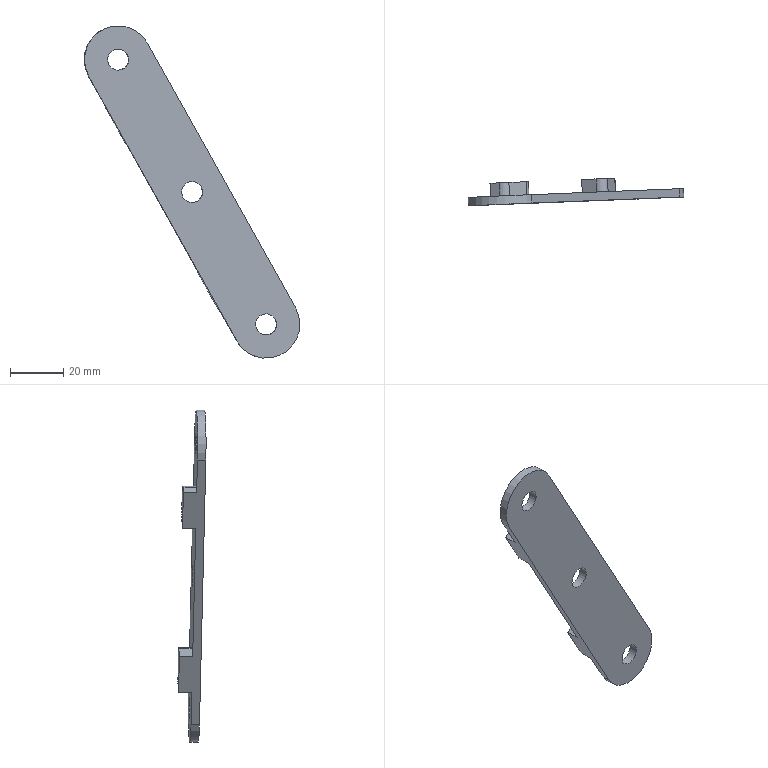Part | NX | features MG0330 trunion parts 24(steering fork) 2 | 1 solid | 21 faces | box 81.261 x 10.57 x 125.154 mm | volume 11578 mm3 | plane 12 | cylinder 9 | commonest cylinder face diameters 6 x4 7.938 x3 25.4 x2
STEP:
#1=CARTESIAN_POINT('',(621.854,-233.442,-30.331));
#2=VERTEX_POINT('',#1);
#3=CARTESIAN_POINT('',(627.267,-233.207,-27.3));
#4=VERTEX_POINT('',#3);
#5=CARTESIAN_POINT('',(621.854,-233.442,-30.331));
#6=DIRECTION('',(0.8719,0.03772,0.4882));
#7=VECTOR('',#6,1000.);
#8=LINE('',#5,#7);
#9=EDGE_CURVE('',#2,#4,#8,.T.);
#10=ORIENTED_EDGE('',*,*,#9,.F.);
#11=CARTESIAN_POINT('',(594.883,-234.609,17.931));
#12=VERTEX_POINT('',#11);
#13=CARTESIAN_POINT('',(636.242,-232.819,-56.077));
#14=DIRECTION('',(-0.4877,-0.0211,0.8727));
#15=VECTOR('',#14,1000.);
#16=LINE('',#13,#15);
#17=EDGE_CURVE('',#2,#12,#16,.T.);
#18=ORIENTED_EDGE('',*,*,#17,.T.);
#19=CARTESIAN_POINT('',(600.295,-234.374,20.962));
#20=VERTEX_POINT('',#19);
#21=CARTESIAN_POINT('',(594.883,-234.609,17.931));
#22=DIRECTION('',(0.8719,0.03772,0.4882));
#23=VECTOR('',#22,1000.);
#24=LINE('',#21,#23);
#25=EDGE_CURVE('',#20,#12,#24,.F.);
#26=ORIENTED_EDGE('',*,*,#25,.F.);
#27=CARTESIAN_POINT('',(601.041,-234.342,25.607));
#28=VERTEX_POINT('',#27);
#29=CARTESIAN_POINT('',(598.832,-234.438,23.58));
#30=DIRECTION('',(0.04322,-0.9991,0.));
#31=DIRECTION('',(-0.4877,-0.0211,0.8727));
#32=AXIS2_PLACEMENT_3D('',#29,#30,#31);
#33=CIRCLE('',#32,3.);
#34=EDGE_CURVE('',#20,#28,#33,.T.);
#35=ORIENTED_EDGE('',*,*,#34,.T.);
#36=CARTESIAN_POINT('',(594.449,-234.627,32.802));
#37=VERTEX_POINT('',#36);
#38=CARTESIAN_POINT('',(603.602,-234.231,22.813));
#39=DIRECTION('',(-0.6753,-0.02921,0.737));
#40=VECTOR('',#39,1000.);
#41=LINE('',#38,#40);
#42=EDGE_CURVE('',#28,#37,#41,.T.);
#43=ORIENTED_EDGE('',*,*,#42,.T.);
#44=CARTESIAN_POINT('',(590.777,-234.786,33.393));
#45=VERTEX_POINT('',#44);
#46=CARTESIAN_POINT('',(592.24,-234.723,30.775));
#47=DIRECTION('',(0.04322,-0.9991,0.));
#48=DIRECTION('',(-0.4877,-0.0211,0.8727));
#49=AXIS2_PLACEMENT_3D('',#46,#47,#48);
#50=CIRCLE('',#49,3.);
#51=EDGE_CURVE('',#37,#45,#50,.T.);
#52=ORIENTED_EDGE('',*,*,#51,.T.);
#53=CARTESIAN_POINT('',(587.322,-234.936,31.459));
#54=VERTEX_POINT('',#53);
#55=CARTESIAN_POINT('',(592.847,-234.697,34.552));
#56=DIRECTION('',(-0.8719,-0.03772,-0.4882));
#57=VECTOR('',#56,1000.);
#58=LINE('',#55,#57);
#59=EDGE_CURVE('',#54,#45,#58,.F.);
#60=ORIENTED_EDGE('',*,*,#59,.F.);
#61=CARTESIAN_POINT('',(580.494,-235.231,43.677));
#62=VERTEX_POINT('',#61);
#63=CARTESIAN_POINT('',(636.242,-232.819,-56.077));
#64=DIRECTION('',(-0.4877,-0.0211,0.8727));
#65=VECTOR('',#64,1000.);
#66=LINE('',#63,#65);
#67=EDGE_CURVE('',#54,#62,#66,.T.);
#68=ORIENTED_EDGE('',*,*,#67,.T.);
#69=CARTESIAN_POINT('',(602.641,-234.273,56.077));
#70=VERTEX_POINT('',#69);
#71=CARTESIAN_POINT('',(591.568,-234.752,49.877));
#72=DIRECTION('',(-0.04322,0.9991,0.));
#73=DIRECTION('',(0.8719,0.03772,0.4882));
#74=AXIS2_PLACEMENT_3D('',#71,#72,#73);
#75=CIRCLE('',#74,12.7);
#76=EDGE_CURVE('',#62,#70,#75,.T.);
#77=ORIENTED_EDGE('',*,*,#76,.T.);
#78=CARTESIAN_POINT('',(658.389,-231.861,-43.677));
#79=VERTEX_POINT('',#78);
#80=CARTESIAN_POINT('',(658.389,-231.861,-43.677));
#81=DIRECTION('',(0.4877,0.0211,-0.8727));
#82=VECTOR('',#81,1000.);
#83=LINE('',#80,#82);
#84=EDGE_CURVE('',#70,#79,#83,.T.);
#85=ORIENTED_EDGE('',*,*,#84,.T.);
#86=CARTESIAN_POINT('',(636.242,-232.819,-56.077));
#87=VERTEX_POINT('',#86);
#88=CARTESIAN_POINT('',(647.315,-232.34,-49.877));
#89=DIRECTION('',(-0.04322,0.9991,0.));
#90=DIRECTION('',(0.8719,0.03772,0.4882));
#91=AXIS2_PLACEMENT_3D('',#88,#89,#90);
#92=CIRCLE('',#91,12.7);
#93=EDGE_CURVE('',#79,#87,#92,.T.);
#94=ORIENTED_EDGE('',*,*,#93,.T.);
#95=CARTESIAN_POINT('',(629.414,-233.115,-43.859));
#96=VERTEX_POINT('',#95);
#97=CARTESIAN_POINT('',(636.242,-232.819,-56.077));
#98=DIRECTION('',(-0.4877,-0.0211,0.8727));
#99=VECTOR('',#98,1000.);
#100=LINE('',#97,#99);
#101=EDGE_CURVE('',#87,#96,#100,.T.);
#102=ORIENTED_EDGE('',*,*,#101,.T.);
#103=CARTESIAN_POINT('',(632.868,-232.965,-41.924));
#104=VERTEX_POINT('',#103);
#105=CARTESIAN_POINT('',(634.938,-232.876,-40.766));
#106=DIRECTION('',(-0.8719,-0.03772,-0.4882));
#107=VECTOR('',#106,1000.);
#108=LINE('',#105,#107);
#109=EDGE_CURVE('',#104,#96,#108,.T.);
#110=ORIENTED_EDGE('',*,*,#109,.F.);
#111=CARTESIAN_POINT('',(634.287,-232.904,-38.483));
#112=VERTEX_POINT('',#111);
#113=CARTESIAN_POINT('',(631.405,-233.028,-39.306));
#114=DIRECTION('',(-0.04322,0.9991,0.));
#115=DIRECTION('',(-0.9991,-0.04322,0.));
#116=AXIS2_PLACEMENT_3D('',#113,#114,#115);
#117=CIRCLE('',#116,3.);
#118=EDGE_CURVE('',#104,#112,#117,.F.);
#119=ORIENTED_EDGE('',*,*,#118,.T.);
#120=CARTESIAN_POINT('',(631.612,-233.019,-29.095));
#121=VERTEX_POINT('',#120);
#122=CARTESIAN_POINT('',(633.424,-232.941,-35.455));
#123=DIRECTION('',(0.274,0.01186,-0.9616));
#124=VECTOR('',#123,1000.);
#125=LINE('',#122,#124);
#126=EDGE_CURVE('',#121,#112,#125,.T.);
#127=ORIENTED_EDGE('',*,*,#126,.F.);
#128=CARTESIAN_POINT('',(628.73,-233.144,-29.918));
#129=DIRECTION('',(-0.04322,0.9991,0.));
#130=DIRECTION('',(-0.9991,-0.04322,0.));
#131=AXIS2_PLACEMENT_3D('',#128,#129,#130);
#132=CIRCLE('',#131,3.);
#133=EDGE_CURVE('',#121,#4,#132,.F.);
#134=ORIENTED_EDGE('',*,*,#133,.T.);
#135=EDGE_LOOP('',(#10,#18,#26,#35,#43,#52,#60,#68,#77,#85,#94,#102,#110,#119,#127,#134));
#136=FACE_BOUND('',#135,.T.);
#137=CARTESIAN_POINT('',(595.028,-234.602,51.814));
#138=VERTEX_POINT('',#137);
#139=CARTESIAN_POINT('',(591.568,-234.752,49.877));
#140=DIRECTION('',(-0.04322,0.9991,0.));
#141=DIRECTION('',(0.8719,0.03772,0.4882));
#142=AXIS2_PLACEMENT_3D('',#139,#140,#141);
#143=CIRCLE('',#142,3.969);
#144=EDGE_CURVE('',#138,#138,#143,.T.);
#145=ORIENTED_EDGE('',*,*,#144,.F.);
#146=EDGE_LOOP('',(#145));
#147=FACE_BOUND('',#146,.T.);
#148=CARTESIAN_POINT('',(622.902,-233.396,1.937));
#149=VERTEX_POINT('',#148);
#150=CARTESIAN_POINT('',(619.442,-233.546,0.));
#151=DIRECTION('',(-0.04322,0.9991,0.));
#152=DIRECTION('',(0.8719,0.03772,0.4882));
#153=AXIS2_PLACEMENT_3D('',#150,#151,#152);
#154=CIRCLE('',#153,3.969);
#155=EDGE_CURVE('',#149,#149,#154,.T.);
#156=ORIENTED_EDGE('',*,*,#155,.F.);
#157=EDGE_LOOP('',(#156));
#158=FACE_BOUND('',#157,.T.);
#159=CARTESIAN_POINT('',(650.776,-232.19,-47.94));
#160=VERTEX_POINT('',#159);
#161=CARTESIAN_POINT('',(647.315,-232.34,-49.877));
#162=DIRECTION('',(-0.04322,0.9991,0.));
#163=DIRECTION('',(0.8719,0.03772,0.4882));
#164=AXIS2_PLACEMENT_3D('',#161,#162,#163);
#165=CIRCLE('',#164,3.969);
#166=EDGE_CURVE('',#160,#160,#165,.T.);
#167=ORIENTED_EDGE('',*,*,#166,.F.);
#168=EDGE_LOOP('',(#167));
#169=FACE_BOUND('',#168,.T.);
#170=CARTESIAN_POINT('',(647.315,-232.34,-49.877));
#171=DIRECTION('',(-0.04322,0.9991,0.));
#172=DIRECTION('',(0.8719,0.03772,0.4882));
#173=AXIS2_PLACEMENT_3D('',#170,#171,#172);
#174=PLANE('',#173);
#175=ADVANCED_FACE('',(#136,#147,#158,#169),#174,.T.);
#176=CARTESIAN_POINT('',(658.526,-235.033,-43.677));
#177=VERTEX_POINT('',#176);
#178=CARTESIAN_POINT('',(636.379,-235.991,-56.077));
#179=VERTEX_POINT('',#178);
#180=CARTESIAN_POINT('',(647.453,-235.512,-49.877));
#181=DIRECTION('',(-0.04322,0.9991,0.));
#182=DIRECTION('',(0.8719,0.03772,0.4882));
#183=AXIS2_PLACEMENT_3D('',#180,#181,#182);
#184=CIRCLE('',#183,12.7);
#185=EDGE_CURVE('',#177,#179,#184,.T.);
#186=ORIENTED_EDGE('',*,*,#185,.F.);
#187=CARTESIAN_POINT('',(602.778,-237.445,56.077));
#188=VERTEX_POINT('',#187);
#189=CARTESIAN_POINT('',(658.526,-235.033,-43.677));
#190=DIRECTION('',(0.4877,0.0211,-0.8727));
#191=VECTOR('',#190,1000.);
#192=LINE('',#189,#191);
#193=EDGE_CURVE('',#188,#177,#192,.T.);
#194=ORIENTED_EDGE('',*,*,#193,.F.);
#195=CARTESIAN_POINT('',(580.631,-238.403,43.677));
#196=VERTEX_POINT('',#195);
#197=CARTESIAN_POINT('',(591.705,-237.924,49.877));
#198=DIRECTION('',(-0.04322,0.9991,0.));
#199=DIRECTION('',(0.8719,0.03772,0.4882));
#200=AXIS2_PLACEMENT_3D('',#197,#198,#199);
#201=CIRCLE('',#200,12.7);
#202=EDGE_CURVE('',#196,#188,#201,.T.);
#203=ORIENTED_EDGE('',*,*,#202,.F.);
#204=CARTESIAN_POINT('',(636.379,-235.991,-56.077));
#205=DIRECTION('',(-0.4877,-0.0211,0.8727));
#206=VECTOR('',#205,1000.);
#207=LINE('',#204,#206);
#208=EDGE_CURVE('',#179,#196,#207,.T.);
#209=ORIENTED_EDGE('',*,*,#208,.F.);
#210=EDGE_LOOP('',(#186,#194,#203,#209));
#211=FACE_BOUND('',#210,.T.);
#212=CARTESIAN_POINT('',(623.039,-236.568,1.937));
#213=VERTEX_POINT('',#212);
#214=CARTESIAN_POINT('',(619.579,-236.718,0.));
#215=DIRECTION('',(-0.04322,0.9991,0.));
#216=DIRECTION('',(0.8719,0.03772,0.4882));
#217=AXIS2_PLACEMENT_3D('',#214,#215,#216);
#218=CIRCLE('',#217,3.969);
#219=EDGE_CURVE('',#213,#213,#218,.T.);
#220=ORIENTED_EDGE('',*,*,#219,.T.);
#221=EDGE_LOOP('',(#220));
#222=FACE_BOUND('',#221,.T.);
#223=CARTESIAN_POINT('',(595.165,-237.774,51.814));
#224=VERTEX_POINT('',#223);
#225=CARTESIAN_POINT('',(591.705,-237.924,49.877));
#226=DIRECTION('',(-0.04322,0.9991,0.));
#227=DIRECTION('',(0.8719,0.03772,0.4882));
#228=AXIS2_PLACEMENT_3D('',#225,#226,#227);
#229=CIRCLE('',#228,3.969);
#230=EDGE_CURVE('',#224,#224,#229,.T.);
#231=ORIENTED_EDGE('',*,*,#230,.T.);
#232=EDGE_LOOP('',(#231));
#233=FACE_BOUND('',#232,.T.);
#234=CARTESIAN_POINT('',(650.913,-235.362,-47.94));
#235=VERTEX_POINT('',#234);
#236=CARTESIAN_POINT('',(647.453,-235.512,-49.877));
#237=DIRECTION('',(-0.04322,0.9991,0.));
#238=DIRECTION('',(0.8719,0.03772,0.4882));
#239=AXIS2_PLACEMENT_3D('',#236,#237,#238);
#240=CIRCLE('',#239,3.969);
#241=EDGE_CURVE('',#235,#235,#240,.T.);
#242=ORIENTED_EDGE('',*,*,#241,.T.);
#243=EDGE_LOOP('',(#242));
#244=FACE_BOUND('',#243,.T.);
#245=CARTESIAN_POINT('',(647.453,-235.512,-49.877));
#246=DIRECTION('',(-0.04322,0.9991,0.));
#247=DIRECTION('',(0.8719,0.03772,0.4882));
#248=AXIS2_PLACEMENT_3D('',#245,#246,#247);
#249=PLANE('',#248);
#250=ADVANCED_FACE('',(#211,#222,#233,#244),#249,.F.);
#251=ORIENTED_EDGE('',*,*,#185,.T.);
#252=CARTESIAN_POINT('',(636.242,-232.819,-56.077));
#253=DIRECTION('',(0.04322,-0.9991,0.));
#254=VECTOR('',#253,1000.);
#255=LINE('',#252,#254);
#256=EDGE_CURVE('',#87,#179,#255,.T.);
#257=ORIENTED_EDGE('',*,*,#256,.F.);
#258=ORIENTED_EDGE('',*,*,#93,.F.);
#259=CARTESIAN_POINT('',(658.389,-231.861,-43.677));
#260=DIRECTION('',(0.04322,-0.9991,0.));
#261=VECTOR('',#260,1000.);
#262=LINE('',#259,#261);
#263=EDGE_CURVE('',#79,#177,#262,.T.);
#264=ORIENTED_EDGE('',*,*,#263,.T.);
#265=EDGE_LOOP('',(#251,#257,#258,#264));
#266=FACE_BOUND('',#265,.T.);
#267=CARTESIAN_POINT('',(647.315,-232.34,-49.877));
#268=DIRECTION('',(0.04322,-0.9991,0.));
#269=DIRECTION('',(-0.8719,-0.03772,-0.4882));
#270=AXIS2_PLACEMENT_3D('',#267,#268,#269);
#271=CYLINDRICAL_SURFACE('',#270,12.7);
#272=ADVANCED_FACE('',(#266),#271,.T.);
#273=ORIENTED_EDGE('',*,*,#208,.T.);
#274=CARTESIAN_POINT('',(580.494,-235.231,43.677));
#275=DIRECTION('',(0.04322,-0.9991,0.));
#276=VECTOR('',#275,1000.);
#277=LINE('',#274,#276);
#278=EDGE_CURVE('',#62,#196,#277,.T.);
#279=ORIENTED_EDGE('',*,*,#278,.F.);
#280=ORIENTED_EDGE('',*,*,#67,.F.);
#281=CARTESIAN_POINT('',(587.106,-229.94,31.459));
#282=VERTEX_POINT('',#281);
#283=CARTESIAN_POINT('',(587.106,-229.94,31.459));
#284=DIRECTION('',(0.04322,-0.9991,0.));
#285=VECTOR('',#284,1000.);
#286=LINE('',#283,#285);
#287=EDGE_CURVE('',#54,#282,#286,.F.);
#288=ORIENTED_EDGE('',*,*,#287,.T.);
#289=CARTESIAN_POINT('',(594.666,-229.613,17.931));
#290=VERTEX_POINT('',#289);
#291=CARTESIAN_POINT('',(587.106,-229.94,31.459));
#292=DIRECTION('',(0.4877,0.0211,-0.8727));
#293=VECTOR('',#292,1000.);
#294=LINE('',#291,#293);
#295=EDGE_CURVE('',#290,#282,#294,.F.);
#296=ORIENTED_EDGE('',*,*,#295,.F.);
#297=CARTESIAN_POINT('',(594.666,-229.613,17.931));
#298=DIRECTION('',(0.04322,-0.9991,0.));
#299=VECTOR('',#298,1000.);
#300=LINE('',#297,#299);
#301=EDGE_CURVE('',#12,#290,#300,.F.);
#302=ORIENTED_EDGE('',*,*,#301,.F.);
#303=ORIENTED_EDGE('',*,*,#17,.F.);
#304=CARTESIAN_POINT('',(621.638,-228.446,-30.331));
#305=VERTEX_POINT('',#304);
#306=CARTESIAN_POINT('',(621.638,-228.446,-30.331));
#307=DIRECTION('',(0.04322,-0.9991,0.));
#308=VECTOR('',#307,1000.);
#309=LINE('',#306,#308);
#310=EDGE_CURVE('',#305,#2,#309,.T.);
#311=ORIENTED_EDGE('',*,*,#310,.F.);
#312=CARTESIAN_POINT('',(629.198,-228.119,-43.859));
#313=VERTEX_POINT('',#312);
#314=CARTESIAN_POINT('',(629.198,-228.119,-43.859));
#315=DIRECTION('',(-0.4877,-0.0211,0.8727));
#316=VECTOR('',#315,1000.);
#317=LINE('',#314,#316);
#318=EDGE_CURVE('',#313,#305,#317,.T.);
#319=ORIENTED_EDGE('',*,*,#318,.F.);
#320=CARTESIAN_POINT('',(629.198,-228.119,-43.859));
#321=DIRECTION('',(0.04322,-0.9991,0.));
#322=VECTOR('',#321,1000.);
#323=LINE('',#320,#322);
#324=EDGE_CURVE('',#313,#96,#323,.T.);
#325=ORIENTED_EDGE('',*,*,#324,.T.);
#326=ORIENTED_EDGE('',*,*,#101,.F.);
#327=ORIENTED_EDGE('',*,*,#256,.T.);
#328=EDGE_LOOP('',(#273,#279,#280,#288,#296,#302,#303,#311,#319,#325,#326,#327));
#329=FACE_BOUND('',#328,.T.);
#330=CARTESIAN_POINT('',(636.242,-232.819,-56.077));
#331=DIRECTION('',(0.8719,0.03772,0.4882));
#332=DIRECTION('',(-0.4877,-0.0211,0.8727));
#333=AXIS2_PLACEMENT_3D('',#330,#331,#332);
#334=PLANE('',#333);
#335=ADVANCED_FACE('',(#329),#334,.F.);
#336=ORIENTED_EDGE('',*,*,#202,.T.);
#337=CARTESIAN_POINT('',(602.641,-234.273,56.077));
#338=DIRECTION('',(0.04322,-0.9991,0.));
#339=VECTOR('',#338,1000.);
#340=LINE('',#337,#339);
#341=EDGE_CURVE('',#70,#188,#340,.T.);
#342=ORIENTED_EDGE('',*,*,#341,.F.);
#343=ORIENTED_EDGE('',*,*,#76,.F.);
#344=ORIENTED_EDGE('',*,*,#278,.T.);
#345=EDGE_LOOP('',(#336,#342,#343,#344));
#346=FACE_BOUND('',#345,.T.);
#347=CARTESIAN_POINT('',(591.568,-234.752,49.877));
#348=DIRECTION('',(0.04322,-0.9991,0.));
#349=DIRECTION('',(-0.8719,-0.03772,-0.4882));
#350=AXIS2_PLACEMENT_3D('',#347,#348,#349);
#351=CYLINDRICAL_SURFACE('',#350,12.7);
#352=ADVANCED_FACE('',(#346),#351,.T.);
#353=ORIENTED_EDGE('',*,*,#193,.T.);
#354=ORIENTED_EDGE('',*,*,#263,.F.);
#355=ORIENTED_EDGE('',*,*,#84,.F.);
#356=ORIENTED_EDGE('',*,*,#341,.T.);
#357=EDGE_LOOP('',(#353,#354,#355,#356));
#358=FACE_BOUND('',#357,.T.);
#359=CARTESIAN_POINT('',(658.389,-231.861,-43.677));
#360=DIRECTION('',(-0.8719,-0.03772,-0.4882));
#361=DIRECTION('',(0.4877,0.0211,-0.8727));
#362=AXIS2_PLACEMENT_3D('',#359,#360,#361);
#363=PLANE('',#362);
#364=ADVANCED_FACE('',(#358),#363,.F.);
#365=ORIENTED_EDGE('',*,*,#155,.T.);
#366=EDGE_LOOP('',(#365));
#367=FACE_BOUND('',#366,.T.);
#368=ORIENTED_EDGE('',*,*,#219,.F.);
#369=EDGE_LOOP('',(#368));
#370=FACE_BOUND('',#369,.T.);
#371=CARTESIAN_POINT('',(619.442,-233.546,0.));
#372=DIRECTION('',(0.04322,-0.9991,0.));
#373=DIRECTION('',(-0.8719,-0.03772,-0.4882));
#374=AXIS2_PLACEMENT_3D('',#371,#372,#373);
#375=CYLINDRICAL_SURFACE('',#374,3.969);
#376=ADVANCED_FACE('',(#367,#370),#375,.F.);
#377=ORIENTED_EDGE('',*,*,#144,.T.);
#378=EDGE_LOOP('',(#377));
#379=FACE_BOUND('',#378,.T.);
#380=ORIENTED_EDGE('',*,*,#230,.F.);
#381=EDGE_LOOP('',(#380));
#382=FACE_BOUND('',#381,.T.);
#383=CARTESIAN_POINT('',(591.568,-234.752,49.877));
#384=DIRECTION('',(0.04322,-0.9991,0.));
#385=DIRECTION('',(-0.8719,-0.03772,-0.4882));
#386=AXIS2_PLACEMENT_3D('',#383,#384,#385);
#387=CYLINDRICAL_SURFACE('',#386,3.969);
#388=ADVANCED_FACE('',(#379,#382),#387,.F.);
#389=ORIENTED_EDGE('',*,*,#166,.T.);
#390=EDGE_LOOP('',(#389));
#391=FACE_BOUND('',#390,.T.);
#392=ORIENTED_EDGE('',*,*,#241,.F.);
#393=EDGE_LOOP('',(#392));
#394=FACE_BOUND('',#393,.T.);
#395=CARTESIAN_POINT('',(647.315,-232.34,-49.877));
#396=DIRECTION('',(0.04322,-0.9991,0.));
#397=DIRECTION('',(-0.8719,-0.03772,-0.4882));
#398=AXIS2_PLACEMENT_3D('',#395,#396,#397);
#399=CYLINDRICAL_SURFACE('',#398,3.969);
#400=ADVANCED_FACE('',(#391,#394),#399,.F.);
#401=CARTESIAN_POINT('',(600.079,-229.379,20.962));
#402=VERTEX_POINT('',#401);
#403=CARTESIAN_POINT('',(594.666,-229.613,17.931));
#404=DIRECTION('',(0.8719,0.03772,0.4882));
#405=VECTOR('',#404,1000.);
#406=LINE('',#403,#405);
#407=EDGE_CURVE('',#402,#290,#406,.F.);
#408=ORIENTED_EDGE('',*,*,#407,.F.);
#409=CARTESIAN_POINT('',(600.079,-229.379,20.962));
#410=DIRECTION('',(0.04322,-0.9991,0.));
#411=VECTOR('',#410,1000.);
#412=LINE('',#409,#411);
#413=EDGE_CURVE('',#402,#20,#412,.T.);
#414=ORIENTED_EDGE('',*,*,#413,.T.);
#415=ORIENTED_EDGE('',*,*,#25,.T.);
#416=ORIENTED_EDGE('',*,*,#301,.T.);
#417=EDGE_LOOP('',(#408,#414,#415,#416));
#418=FACE_BOUND('',#417,.T.);
#419=CARTESIAN_POINT('',(594.666,-229.613,17.931));
#420=DIRECTION('',(0.4877,0.0211,-0.8727));
#421=DIRECTION('',(-0.8729,0.,-0.4878));
#422=AXIS2_PLACEMENT_3D('',#419,#420,#421);
#423=PLANE('',#422);
#424=ADVANCED_FACE('',(#418),#423,.T.);
#425=CARTESIAN_POINT('',(600.825,-229.347,25.607));
#426=VERTEX_POINT('',#425);
#427=CARTESIAN_POINT('',(594.233,-229.632,32.802));
#428=VERTEX_POINT('',#427);
#429=CARTESIAN_POINT('',(603.386,-229.236,22.813));
#430=DIRECTION('',(-0.6753,-0.02921,0.737));
#431=VECTOR('',#430,1000.);
#432=LINE('',#429,#431);
#433=EDGE_CURVE('',#426,#428,#432,.T.);
#434=ORIENTED_EDGE('',*,*,#433,.T.);
#435=CARTESIAN_POINT('',(594.233,-229.632,32.802));
#436=DIRECTION('',(0.04322,-0.9991,0.));
#437=VECTOR('',#436,1000.);
#438=LINE('',#435,#437);
#439=EDGE_CURVE('',#428,#37,#438,.T.);
#440=ORIENTED_EDGE('',*,*,#439,.T.);
#441=ORIENTED_EDGE('',*,*,#42,.F.);
#442=CARTESIAN_POINT('',(600.825,-229.347,25.607));
#443=DIRECTION('',(0.04322,-0.9991,0.));
#444=VECTOR('',#443,1000.);
#445=LINE('',#442,#444);
#446=EDGE_CURVE('',#28,#426,#445,.F.);
#447=ORIENTED_EDGE('',*,*,#446,.T.);
#448=EDGE_LOOP('',(#434,#440,#441,#447));
#449=FACE_BOUND('',#448,.T.);
#450=CARTESIAN_POINT('',(603.386,-229.236,22.813));
#451=DIRECTION('',(0.7363,0.03186,0.6759));
#452=DIRECTION('',(0.6762,0.,-0.7367));
#453=AXIS2_PLACEMENT_3D('',#450,#451,#452);
#454=PLANE('',#453);
#455=ADVANCED_FACE('',(#449),#454,.T.);
#456=ORIENTED_EDGE('',*,*,#59,.T.);
#457=CARTESIAN_POINT('',(590.561,-229.791,33.393));
#458=VERTEX_POINT('',#457);
#459=CARTESIAN_POINT('',(590.561,-229.791,33.393));
#460=DIRECTION('',(0.04322,-0.9991,0.));
#461=VECTOR('',#460,1000.);
#462=LINE('',#459,#461);
#463=EDGE_CURVE('',#45,#458,#462,.F.);
#464=ORIENTED_EDGE('',*,*,#463,.T.);
#465=CARTESIAN_POINT('',(592.63,-229.701,34.552));
#466=DIRECTION('',(-0.8719,-0.03772,-0.4882));
#467=VECTOR('',#466,1000.);
#468=LINE('',#465,#467);
#469=EDGE_CURVE('',#282,#458,#468,.F.);
#470=ORIENTED_EDGE('',*,*,#469,.F.);
#471=ORIENTED_EDGE('',*,*,#287,.F.);
#472=EDGE_LOOP('',(#456,#464,#470,#471));
#473=FACE_BOUND('',#472,.T.);
#474=CARTESIAN_POINT('',(592.63,-229.701,34.552));
#475=DIRECTION('',(-0.4877,-0.0211,0.8727));
#476=DIRECTION('',(0.8729,0.,0.4878));
#477=AXIS2_PLACEMENT_3D('',#474,#475,#476);
#478=PLANE('',#477);
#479=ADVANCED_FACE('',(#473),#478,.T.);
#480=ORIENTED_EDGE('',*,*,#469,.T.);
#481=CARTESIAN_POINT('',(592.024,-229.727,30.775));
#482=DIRECTION('',(0.04322,-0.9991,0.));
#483=DIRECTION('',(-0.4877,-0.0211,0.8727));
#484=AXIS2_PLACEMENT_3D('',#481,#482,#483);
#485=CIRCLE('',#484,3.);
#486=EDGE_CURVE('',#458,#428,#485,.F.);
#487=ORIENTED_EDGE('',*,*,#486,.T.);
#488=ORIENTED_EDGE('',*,*,#433,.F.);
#489=CARTESIAN_POINT('',(598.616,-229.442,23.58));
#490=DIRECTION('',(0.04322,-0.9991,0.));
#491=DIRECTION('',(-0.4877,-0.0211,0.8727));
#492=AXIS2_PLACEMENT_3D('',#489,#490,#491);
#493=CIRCLE('',#492,3.);
#494=EDGE_CURVE('',#426,#402,#493,.F.);
#495=ORIENTED_EDGE('',*,*,#494,.T.);
#496=ORIENTED_EDGE('',*,*,#407,.T.);
#497=ORIENTED_EDGE('',*,*,#295,.T.);
#498=EDGE_LOOP('',(#480,#487,#488,#495,#496,#497));
#499=FACE_BOUND('',#498,.T.);
#500=CARTESIAN_POINT('',(11.027,-254.864,0.));
#501=DIRECTION('',(0.04322,-0.9991,0.));
#502=DIRECTION('',(0.9991,0.04322,0.));
#503=AXIS2_PLACEMENT_3D('',#500,#501,#502);
#504=PLANE('',#503);
#505=ADVANCED_FACE('',(#499),#504,.F.);
#506=ORIENTED_EDGE('',*,*,#486,.F.);
#507=ORIENTED_EDGE('',*,*,#463,.F.);
#508=ORIENTED_EDGE('',*,*,#51,.F.);
#509=ORIENTED_EDGE('',*,*,#439,.F.);
#510=EDGE_LOOP('',(#506,#507,#508,#509));
#511=FACE_BOUND('',#510,.T.);
#512=CARTESIAN_POINT('',(592.024,-229.727,30.775));
#513=DIRECTION('',(0.04322,-0.9991,0.));
#514=DIRECTION('',(-0.4877,-0.0211,0.8727));
#515=AXIS2_PLACEMENT_3D('',#512,#513,#514);
#516=CYLINDRICAL_SURFACE('',#515,3.);
#517=ADVANCED_FACE('',(#511),#516,.T.);
#518=ORIENTED_EDGE('',*,*,#494,.F.);
#519=ORIENTED_EDGE('',*,*,#446,.F.);
#520=ORIENTED_EDGE('',*,*,#34,.F.);
#521=ORIENTED_EDGE('',*,*,#413,.F.);
#522=EDGE_LOOP('',(#518,#519,#520,#521));
#523=FACE_BOUND('',#522,.T.);
#524=CARTESIAN_POINT('',(598.616,-229.442,23.58));
#525=DIRECTION('',(0.04322,-0.9991,0.));
#526=DIRECTION('',(-0.4877,-0.0211,0.8727));
#527=AXIS2_PLACEMENT_3D('',#524,#525,#526);
#528=CYLINDRICAL_SURFACE('',#527,3.);
#529=ADVANCED_FACE('',(#523),#528,.T.);
#530=ORIENTED_EDGE('',*,*,#9,.T.);
#531=CARTESIAN_POINT('',(627.05,-228.212,-27.3));
#532=VERTEX_POINT('',#531);
#533=CARTESIAN_POINT('',(627.05,-228.212,-27.3));
#534=DIRECTION('',(0.04322,-0.9991,0.));
#535=VECTOR('',#534,1000.);
#536=LINE('',#533,#535);
#537=EDGE_CURVE('',#4,#532,#536,.F.);
#538=ORIENTED_EDGE('',*,*,#537,.T.);
#539=CARTESIAN_POINT('',(621.638,-228.446,-30.331));
#540=DIRECTION('',(0.8719,0.03772,0.4882));
#541=VECTOR('',#540,1000.);
#542=LINE('',#539,#541);
#543=EDGE_CURVE('',#305,#532,#542,.T.);
#544=ORIENTED_EDGE('',*,*,#543,.F.);
#545=ORIENTED_EDGE('',*,*,#310,.T.);
#546=EDGE_LOOP('',(#530,#538,#544,#545));
#547=FACE_BOUND('',#546,.T.);
#548=CARTESIAN_POINT('',(621.638,-228.446,-30.331));
#549=DIRECTION('',(0.4877,0.0211,-0.8727));
#550=DIRECTION('',(-0.8729,0.,-0.4878));
#551=AXIS2_PLACEMENT_3D('',#548,#549,#550);
#552=PLANE('',#551);
#553=ADVANCED_FACE('',(#547),#552,.F.);
#554=CARTESIAN_POINT('',(631.396,-228.024,-29.095));
#555=VERTEX_POINT('',#554);
#556=CARTESIAN_POINT('',(634.071,-227.908,-38.483));
#557=VERTEX_POINT('',#556);
#558=CARTESIAN_POINT('',(630.357,-228.069,-25.449));
#559=DIRECTION('',(0.274,0.01186,-0.9616));
#560=VECTOR('',#559,1000.);
#561=LINE('',#558,#560);
#562=EDGE_CURVE('',#555,#557,#561,.T.);
#563=ORIENTED_EDGE('',*,*,#562,.F.);
#564=CARTESIAN_POINT('',(631.396,-228.024,-29.095));
#565=DIRECTION('',(0.04322,-0.9991,0.));
#566=VECTOR('',#565,1000.);
#567=LINE('',#564,#566);
#568=EDGE_CURVE('',#555,#121,#567,.T.);
#569=ORIENTED_EDGE('',*,*,#568,.T.);
#570=ORIENTED_EDGE('',*,*,#126,.T.);
#571=CARTESIAN_POINT('',(634.071,-227.908,-38.483));
#572=DIRECTION('',(0.04322,-0.9991,0.));
#573=VECTOR('',#572,1000.);
#574=LINE('',#571,#573);
#575=EDGE_CURVE('',#112,#557,#574,.F.);
#576=ORIENTED_EDGE('',*,*,#575,.T.);
#577=EDGE_LOOP('',(#563,#569,#570,#576));
#578=FACE_BOUND('',#577,.T.);
#579=CARTESIAN_POINT('',(633.208,-227.946,-35.455));
#580=DIRECTION('',(-0.9607,-0.04157,-0.2743));
#581=DIRECTION('',(-0.2745,0.,0.9616));
#582=AXIS2_PLACEMENT_3D('',#579,#580,#581);
#583=PLANE('',#582);
#584=ADVANCED_FACE('',(#578),#583,.F.);
#585=CARTESIAN_POINT('',(632.652,-227.97,-41.924));
#586=VERTEX_POINT('',#585);
#587=CARTESIAN_POINT('',(634.722,-227.88,-40.766));
#588=DIRECTION('',(-0.8719,-0.03772,-0.4882));
#589=VECTOR('',#588,1000.);
#590=LINE('',#587,#589);
#591=EDGE_CURVE('',#586,#313,#590,.T.);
#592=ORIENTED_EDGE('',*,*,#591,.F.);
#593=CARTESIAN_POINT('',(632.652,-227.97,-41.924));
#594=DIRECTION('',(0.04322,-0.9991,0.));
#595=VECTOR('',#594,1000.);
#596=LINE('',#593,#595);
#597=EDGE_CURVE('',#586,#104,#596,.T.);
#598=ORIENTED_EDGE('',*,*,#597,.T.);
#599=ORIENTED_EDGE('',*,*,#109,.T.);
#600=ORIENTED_EDGE('',*,*,#324,.F.);
#601=EDGE_LOOP('',(#592,#598,#599,#600));
#602=FACE_BOUND('',#601,.T.);
#603=CARTESIAN_POINT('',(634.722,-227.88,-40.766));
#604=DIRECTION('',(-0.4877,-0.0211,0.8727));
#605=DIRECTION('',(0.8729,0.,0.4878));
#606=AXIS2_PLACEMENT_3D('',#603,#604,#605);
#607=PLANE('',#606);
#608=ADVANCED_FACE('',(#602),#607,.F.);
#609=ORIENTED_EDGE('',*,*,#543,.T.);
#610=CARTESIAN_POINT('',(628.514,-228.149,-29.918));
#611=DIRECTION('',(-0.04322,0.9991,0.));
#612=DIRECTION('',(-0.9991,-0.04322,0.));
#613=AXIS2_PLACEMENT_3D('',#610,#611,#612);
#614=CIRCLE('',#613,3.);
#615=EDGE_CURVE('',#532,#555,#614,.T.);
#616=ORIENTED_EDGE('',*,*,#615,.T.);
#617=ORIENTED_EDGE('',*,*,#562,.T.);
#618=CARTESIAN_POINT('',(631.189,-228.033,-39.306));
#619=DIRECTION('',(-0.04322,0.9991,0.));
#620=DIRECTION('',(-0.9991,-0.04322,0.));
#621=AXIS2_PLACEMENT_3D('',#618,#619,#620);
#622=CIRCLE('',#621,3.);
#623=EDGE_CURVE('',#557,#586,#622,.T.);
#624=ORIENTED_EDGE('',*,*,#623,.T.);
#625=ORIENTED_EDGE('',*,*,#591,.T.);
#626=ORIENTED_EDGE('',*,*,#318,.T.);
#627=EDGE_LOOP('',(#609,#616,#617,#624,#625,#626));
#628=FACE_BOUND('',#627,.T.);
#629=CARTESIAN_POINT('',(11.027,-254.864,0.));
#630=DIRECTION('',(-0.04322,0.9991,0.));
#631=DIRECTION('',(-0.9991,-0.04322,0.));
#632=AXIS2_PLACEMENT_3D('',#629,#630,#631);
#633=PLANE('',#632);
#634=ADVANCED_FACE('',(#628),#633,.T.);
#635=ORIENTED_EDGE('',*,*,#615,.F.);
#636=ORIENTED_EDGE('',*,*,#537,.F.);
#637=ORIENTED_EDGE('',*,*,#133,.F.);
#638=ORIENTED_EDGE('',*,*,#568,.F.);
#639=EDGE_LOOP('',(#635,#636,#637,#638));
#640=FACE_BOUND('',#639,.T.);
#641=CARTESIAN_POINT('',(628.514,-228.149,-29.918));
#642=DIRECTION('',(0.04322,-0.9991,0.));
#643=DIRECTION('',(0.9991,0.04322,0.));
#644=AXIS2_PLACEMENT_3D('',#641,#642,#643);
#645=CYLINDRICAL_SURFACE('',#644,3.);
#646=ADVANCED_FACE('',(#640),#645,.T.);
#647=ORIENTED_EDGE('',*,*,#623,.F.);
#648=ORIENTED_EDGE('',*,*,#575,.F.);
#649=ORIENTED_EDGE('',*,*,#118,.F.);
#650=ORIENTED_EDGE('',*,*,#597,.F.);
#651=EDGE_LOOP('',(#647,#648,#649,#650));
#652=FACE_BOUND('',#651,.T.);
#653=CARTESIAN_POINT('',(631.189,-228.033,-39.306));
#654=DIRECTION('',(0.04322,-0.9991,0.));
#655=DIRECTION('',(0.9991,0.04322,0.));
#656=AXIS2_PLACEMENT_3D('',#653,#654,#655);
#657=CYLINDRICAL_SURFACE('',#656,3.);
#658=ADVANCED_FACE('',(#652),#657,.T.);
#659=CLOSED_SHELL('',(#175,#250,#272,#335,#352,#364,#376,#388,#400,#424,#455,#479,#505,#517,#529,#553,#584,#608,#634,#646,#658));
#660=MANIFOLD_SOLID_BREP('',#659);
#661=(LENGTH_UNIT()NAMED_UNIT(*)SI_UNIT(.MILLI.,.METRE.));
#662=UNCERTAINTY_MEASURE_WITH_UNIT(LENGTH_MEASURE(0.00001),#661,'','');
#663=(NAMED_UNIT(*)PLANE_ANGLE_UNIT()SI_UNIT($,.RADIAN.));
#664=(NAMED_UNIT(*)SI_UNIT($,.STERADIAN.)SOLID_ANGLE_UNIT());
#665=(GEOMETRIC_REPRESENTATION_CONTEXT(3)GLOBAL_UNCERTAINTY_ASSIGNED_CONTEXT((#662))GLOBAL_UNIT_ASSIGNED_CONTEXT((#661,#663,#664))REPRESENTATION_CONTEXT('',''));
#666=ADVANCED_BREP_SHAPE_REPRESENTATION('',(#660),#665);